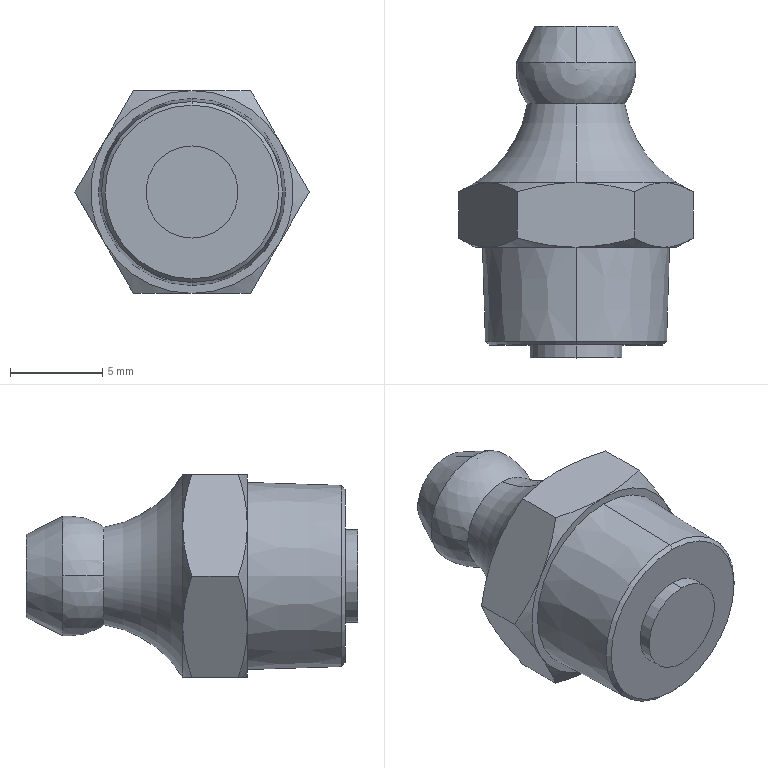Part | SolidWorks | features ICE 9, Revolution 9, Fillet 2 | 2 solids | 43 faces | box 12.702 x 18 x 11 mm | volume 1039 mm3 | cone 20 | plane 11 | cylinder 6 | sphere 4 | torus 2 | commonest cylinder face diameters 1.5 x2 3 x2 5 x2
STEP:
#1=CARTESIAN_POINT('',(0.,13.773,-2.65));
#2=VERTEX_POINT('',#1);
#3=CARTESIAN_POINT('',(-2.65,13.773,0.));
#4=VERTEX_POINT('',#3);
#5=CARTESIAN_POINT('',(0.,13.773,0.));
#6=DIRECTION('',(0.,1.,0.));
#7=DIRECTION('',(0.,0.,1.));
#8=AXIS2_PLACEMENT_3D('',#5,#6,#7);
#9=CIRCLE('',#8,2.65);
#10=EDGE_CURVE('',#2,#4,#9,.T.);
#11=ORIENTED_EDGE('',*,*,#10,.T.);
#12=CARTESIAN_POINT('',(-3.232,16.,0.));
#13=VERTEX_POINT('',#12);
#14=CARTESIAN_POINT('',(0.,15.655,0.));
#15=DIRECTION('',(0.,0.,-1.));
#16=DIRECTION('',(-1.,0.,0.));
#17=AXIS2_PLACEMENT_3D('',#14,#15,#16);
#18=CIRCLE('',#17,3.25);
#19=EDGE_CURVE('',#4,#13,#18,.T.);
#20=ORIENTED_EDGE('',*,*,#19,.T.);
#21=CARTESIAN_POINT('',(0.,16.,-3.232));
#22=VERTEX_POINT('',#21);
#23=CARTESIAN_POINT('',(0.,16.,0.));
#24=DIRECTION('',(0.,1.,0.));
#25=DIRECTION('',(0.,0.,1.));
#26=AXIS2_PLACEMENT_3D('',#23,#24,#25);
#27=CIRCLE('',#26,3.232);
#28=EDGE_CURVE('',#22,#13,#27,.T.);
#29=ORIENTED_EDGE('',*,*,#28,.F.);
#30=CARTESIAN_POINT('',(3.232,16.,0.));
#31=VERTEX_POINT('',#30);
#32=CARTESIAN_POINT('',(0.,16.,0.));
#33=DIRECTION('',(0.,1.,0.));
#34=DIRECTION('',(0.,0.,1.));
#35=AXIS2_PLACEMENT_3D('',#32,#33,#34);
#36=CIRCLE('',#35,3.232);
#37=EDGE_CURVE('',#31,#22,#36,.T.);
#38=ORIENTED_EDGE('',*,*,#37,.F.);
#39=CARTESIAN_POINT('',(2.65,13.773,0.));
#40=VERTEX_POINT('',#39);
#41=CARTESIAN_POINT('',(0.,15.655,0.));
#42=DIRECTION('',(0.,0.,1.));
#43=DIRECTION('',(1.,0.,0.));
#44=AXIS2_PLACEMENT_3D('',#41,#42,#43);
#45=CIRCLE('',#44,3.25);
#46=EDGE_CURVE('',#40,#31,#45,.T.);
#47=ORIENTED_EDGE('',*,*,#46,.F.);
#48=CARTESIAN_POINT('',(0.,13.773,0.));
#49=DIRECTION('',(0.,1.,0.));
#50=DIRECTION('',(0.,0.,1.));
#51=AXIS2_PLACEMENT_3D('',#48,#49,#50);
#52=CIRCLE('',#51,2.65);
#53=EDGE_CURVE('',#40,#2,#52,.T.);
#54=ORIENTED_EDGE('',*,*,#53,.T.);
#55=EDGE_LOOP('',(#11,#20,#29,#38,#47,#54));
#56=FACE_OUTER_BOUND('',#55,.T.);
#57=CARTESIAN_POINT('',(0.,15.655,0.));
#58=DIRECTION('',(0.,0.,-1.));
#59=DIRECTION('',(1.,0.,0.));
#60=AXIS2_PLACEMENT_3D('',#57,#58,#59);
#61=SPHERICAL_SURFACE('',#60,3.25);
#62=ADVANCED_FACE('',(#56),#61,.T.);
#63=CARTESIAN_POINT('',(0.,18.,2.25));
#64=VERTEX_POINT('',#63);
#65=CARTESIAN_POINT('',(0.,18.,-2.25));
#66=VERTEX_POINT('',#65);
#67=CARTESIAN_POINT('',(0.,18.,0.));
#68=DIRECTION('',(0.,1.,0.));
#69=DIRECTION('',(0.,0.,1.));
#70=AXIS2_PLACEMENT_3D('',#67,#68,#69);
#71=CIRCLE('',#70,2.25);
#72=EDGE_CURVE('',#64,#66,#71,.T.);
#73=ORIENTED_EDGE('',*,*,#72,.F.);
#74=CARTESIAN_POINT('',(0.,16.,3.232));
#75=VERTEX_POINT('',#74);
#76=CARTESIAN_POINT('',(0.,18.,2.25));
#77=DIRECTION('',(0.,-0.8977,0.4406));
#78=VECTOR('',#77,1000.);
#79=LINE('',#76,#78);
#80=EDGE_CURVE('',#64,#75,#79,.T.);
#81=ORIENTED_EDGE('',*,*,#80,.T.);
#82=CARTESIAN_POINT('',(0.,16.,0.));
#83=DIRECTION('',(0.,1.,0.));
#84=DIRECTION('',(0.,0.,1.));
#85=AXIS2_PLACEMENT_3D('',#82,#83,#84);
#86=CIRCLE('',#85,3.232);
#87=EDGE_CURVE('',#75,#31,#86,.T.);
#88=ORIENTED_EDGE('',*,*,#87,.T.);
#89=ORIENTED_EDGE('',*,*,#37,.T.);
#90=CARTESIAN_POINT('',(0.,18.,-2.25));
#91=DIRECTION('',(0.,-0.8977,-0.4406));
#92=VECTOR('',#91,1000.);
#93=LINE('',#90,#92);
#94=EDGE_CURVE('',#66,#22,#93,.T.);
#95=ORIENTED_EDGE('',*,*,#94,.F.);
#96=EDGE_LOOP('',(#73,#81,#88,#89,#95));
#97=FACE_OUTER_BOUND('',#96,.T.);
#98=CARTESIAN_POINT('',(0.,18.,0.));
#99=DIRECTION('',(0.,-1.,0.));
#100=DIRECTION('',(0.,0.,-1.));
#101=AXIS2_PLACEMENT_3D('',#98,#99,#100);
#102=CONICAL_SURFACE('',#101,2.25,0.4563);
#103=ADVANCED_FACE('',(#97),#102,.T.);
#104=CARTESIAN_POINT('',(0.,17.689,-0.75));
#105=VERTEX_POINT('',#104);
#106=CARTESIAN_POINT('',(0.,17.689,0.75));
#107=VERTEX_POINT('',#106);
#108=CARTESIAN_POINT('',(0.,17.689,0.));
#109=DIRECTION('',(0.,1.,0.));
#110=DIRECTION('',(0.,0.,1.));
#111=AXIS2_PLACEMENT_3D('',#108,#109,#110);
#112=CIRCLE('',#111,0.75);
#113=EDGE_CURVE('',#105,#107,#112,.T.);
#114=ORIENTED_EDGE('',*,*,#113,.F.);
#115=CARTESIAN_POINT('',(0.,18.,-0.75));
#116=VERTEX_POINT('',#115);
#117=CARTESIAN_POINT('',(0.,18.,-0.75));
#118=DIRECTION('',(0.,1.,0.));
#119=VECTOR('',#118,1000.);
#120=LINE('',#117,#119);
#121=EDGE_CURVE('',#105,#116,#120,.T.);
#122=ORIENTED_EDGE('',*,*,#121,.T.);
#123=CARTESIAN_POINT('',(0.,18.,0.75));
#124=VERTEX_POINT('',#123);
#125=CARTESIAN_POINT('',(0.,18.,0.));
#126=DIRECTION('',(0.,1.,0.));
#127=DIRECTION('',(0.,0.,1.));
#128=AXIS2_PLACEMENT_3D('',#125,#126,#127);
#129=CIRCLE('',#128,0.75);
#130=EDGE_CURVE('',#116,#124,#129,.T.);
#131=ORIENTED_EDGE('',*,*,#130,.T.);
#132=CARTESIAN_POINT('',(0.,18.,0.75));
#133=DIRECTION('',(0.,1.,0.));
#134=VECTOR('',#133,1000.);
#135=LINE('',#132,#134);
#136=EDGE_CURVE('',#107,#124,#135,.T.);
#137=ORIENTED_EDGE('',*,*,#136,.F.);
#138=EDGE_LOOP('',(#114,#122,#131,#137));
#139=FACE_OUTER_BOUND('',#138,.T.);
#140=CARTESIAN_POINT('',(0.,18.,0.));
#141=DIRECTION('',(0.,1.,0.));
#142=DIRECTION('',(0.,0.,1.));
#143=AXIS2_PLACEMENT_3D('',#140,#141,#142);
#144=CYLINDRICAL_SURFACE('',#143,0.75);
#145=ADVANCED_FACE('',(#139),#144,.F.);
#146=ORIENTED_EDGE('',*,*,#113,.T.);
#147=CARTESIAN_POINT('',(0.,16.939,1.5));
#148=VERTEX_POINT('',#147);
#149=CARTESIAN_POINT('',(0.,16.939,1.5));
#150=DIRECTION('',(0.,-0.7071,0.7071));
#151=VECTOR('',#150,1000.);
#152=LINE('',#149,#151);
#153=EDGE_CURVE('',#107,#148,#152,.T.);
#154=ORIENTED_EDGE('',*,*,#153,.T.);
#155=CARTESIAN_POINT('',(0.,16.939,-1.5));
#156=VERTEX_POINT('',#155);
#157=CARTESIAN_POINT('',(0.,16.939,0.));
#158=DIRECTION('',(0.,1.,0.));
#159=DIRECTION('',(0.,0.,1.));
#160=AXIS2_PLACEMENT_3D('',#157,#158,#159);
#161=CIRCLE('',#160,1.5);
#162=EDGE_CURVE('',#156,#148,#161,.T.);
#163=ORIENTED_EDGE('',*,*,#162,.F.);
#164=CARTESIAN_POINT('',(0.,16.939,-1.5));
#165=DIRECTION('',(0.,-0.7071,-0.7071));
#166=VECTOR('',#165,1000.);
#167=LINE('',#164,#166);
#168=EDGE_CURVE('',#105,#156,#167,.T.);
#169=ORIENTED_EDGE('',*,*,#168,.F.);
#170=EDGE_LOOP('',(#146,#154,#163,#169));
#171=FACE_OUTER_BOUND('',#170,.T.);
#172=CARTESIAN_POINT('',(0.,16.939,0.));
#173=DIRECTION('',(0.,-1.,0.));
#174=DIRECTION('',(0.,0.,-1.));
#175=AXIS2_PLACEMENT_3D('',#172,#173,#174);
#176=CONICAL_SURFACE('',#175,1.5,0.7854);
#177=ADVANCED_FACE('',(#171),#176,.F.);
#178=CARTESIAN_POINT('',(0.,9.5,-1.5));
#179=VERTEX_POINT('',#178);
#180=CARTESIAN_POINT('',(0.,9.5,1.5));
#181=VERTEX_POINT('',#180);
#182=CARTESIAN_POINT('',(0.,9.5,0.));
#183=DIRECTION('',(0.,1.,0.));
#184=DIRECTION('',(0.,0.,1.));
#185=AXIS2_PLACEMENT_3D('',#182,#183,#184);
#186=CIRCLE('',#185,1.5);
#187=EDGE_CURVE('',#179,#181,#186,.T.);
#188=ORIENTED_EDGE('',*,*,#187,.F.);
#189=CARTESIAN_POINT('',(0.,18.,-1.5));
#190=DIRECTION('',(0.,1.,0.));
#191=VECTOR('',#190,1000.);
#192=LINE('',#189,#191);
#193=EDGE_CURVE('',#179,#156,#192,.T.);
#194=ORIENTED_EDGE('',*,*,#193,.T.);
#195=ORIENTED_EDGE('',*,*,#162,.T.);
#196=CARTESIAN_POINT('',(0.,18.,1.5));
#197=DIRECTION('',(0.,1.,0.));
#198=VECTOR('',#197,1000.);
#199=LINE('',#196,#198);
#200=EDGE_CURVE('',#181,#148,#199,.T.);
#201=ORIENTED_EDGE('',*,*,#200,.F.);
#202=EDGE_LOOP('',(#188,#194,#195,#201));
#203=FACE_OUTER_BOUND('',#202,.T.);
#204=CARTESIAN_POINT('',(0.,18.,0.));
#205=DIRECTION('',(0.,1.,0.));
#206=DIRECTION('',(0.,0.,1.));
#207=AXIS2_PLACEMENT_3D('',#204,#205,#206);
#208=CYLINDRICAL_SURFACE('',#207,1.5);
#209=ADVANCED_FACE('',(#203),#208,.F.);
#210=ORIENTED_EDGE('',*,*,#10,.F.);
#211=CARTESIAN_POINT('',(0.,9.5,-5.5));
#212=VERTEX_POINT('',#211);
#213=CARTESIAN_POINT('',(0.,14.7,-8.668));
#214=DIRECTION('',(1.,0.,0.));
#215=DIRECTION('',(0.,0.,-1.));
#216=AXIS2_PLACEMENT_3D('',#213,#214,#215);
#217=CIRCLE('',#216,6.089);
#218=EDGE_CURVE('',#2,#212,#217,.T.);
#219=ORIENTED_EDGE('',*,*,#218,.T.);
#220=CARTESIAN_POINT('',(-4.763,9.5,-2.75));
#221=VERTEX_POINT('',#220);
#222=CARTESIAN_POINT('',(0.,9.5,0.));
#223=DIRECTION('',(0.,-1.,0.));
#224=DIRECTION('',(0.,0.,-1.));
#225=AXIS2_PLACEMENT_3D('',#222,#223,#224);
#226=CIRCLE('',#225,5.5);
#227=EDGE_CURVE('',#221,#212,#226,.T.);
#228=ORIENTED_EDGE('',*,*,#227,.F.);
#229=CARTESIAN_POINT('',(-4.763,9.5,2.75));
#230=VERTEX_POINT('',#229);
#231=CARTESIAN_POINT('',(0.,9.5,0.));
#232=DIRECTION('',(0.,-1.,0.));
#233=DIRECTION('',(0.,0.,-1.));
#234=AXIS2_PLACEMENT_3D('',#231,#232,#233);
#235=CIRCLE('',#234,5.5);
#236=EDGE_CURVE('',#230,#221,#235,.T.);
#237=ORIENTED_EDGE('',*,*,#236,.F.);
#238=CARTESIAN_POINT('',(0.,9.5,5.5));
#239=VERTEX_POINT('',#238);
#240=CARTESIAN_POINT('',(0.,9.5,0.));
#241=DIRECTION('',(0.,-1.,0.));
#242=DIRECTION('',(0.,0.,-1.));
#243=AXIS2_PLACEMENT_3D('',#240,#241,#242);
#244=CIRCLE('',#243,5.5);
#245=EDGE_CURVE('',#239,#230,#244,.T.);
#246=ORIENTED_EDGE('',*,*,#245,.F.);
#247=CARTESIAN_POINT('',(0.,13.773,2.65));
#248=VERTEX_POINT('',#247);
#249=CARTESIAN_POINT('',(0.,14.7,8.668));
#250=DIRECTION('',(-1.,0.,0.));
#251=DIRECTION('',(0.,0.,1.));
#252=AXIS2_PLACEMENT_3D('',#249,#250,#251);
#253=CIRCLE('',#252,6.089);
#254=EDGE_CURVE('',#248,#239,#253,.T.);
#255=ORIENTED_EDGE('',*,*,#254,.F.);
#256=CARTESIAN_POINT('',(0.,13.773,0.));
#257=DIRECTION('',(0.,1.,0.));
#258=DIRECTION('',(0.,0.,1.));
#259=AXIS2_PLACEMENT_3D('',#256,#257,#258);
#260=CIRCLE('',#259,2.65);
#261=EDGE_CURVE('',#4,#248,#260,.T.);
#262=ORIENTED_EDGE('',*,*,#261,.F.);
#263=EDGE_LOOP('',(#210,#219,#228,#237,#246,#255,#262));
#264=FACE_OUTER_BOUND('',#263,.T.);
#265=CARTESIAN_POINT('',(0.,14.7,0.));
#266=DIRECTION('',(0.,1.,0.));
#267=DIRECTION('',(0.,0.,1.));
#268=AXIS2_PLACEMENT_3D('',#265,#266,#267);
#269=TOROIDAL_SURFACE('',#268,8.668,6.089);
#270=ADVANCED_FACE('',(#264),#269,.F.);
#271=CARTESIAN_POINT('',(0.,0.9,-4.913));
#272=VERTEX_POINT('',#271);
#273=CARTESIAN_POINT('',(0.,0.9,4.913));
#274=VERTEX_POINT('',#273);
#275=CARTESIAN_POINT('',(0.,0.9,0.));
#276=DIRECTION('',(0.,-1.,0.));
#277=DIRECTION('',(0.,0.,-1.));
#278=AXIS2_PLACEMENT_3D('',#275,#276,#277);
#279=CIRCLE('',#278,4.913);
#280=EDGE_CURVE('',#272,#274,#279,.T.);
#281=ORIENTED_EDGE('',*,*,#280,.F.);
#282=CARTESIAN_POINT('',(0.,6.,-5.072));
#283=VERTEX_POINT('',#282);
#284=CARTESIAN_POINT('',(0.,6.,-5.072));
#285=DIRECTION('',(0.,0.9995,-0.03123));
#286=VECTOR('',#285,1000.);
#287=LINE('',#284,#286);
#288=EDGE_CURVE('',#272,#283,#287,.T.);
#289=ORIENTED_EDGE('',*,*,#288,.T.);
#290=CARTESIAN_POINT('',(0.,6.,5.072));
#291=VERTEX_POINT('',#290);
#292=CARTESIAN_POINT('',(0.,6.,0.));
#293=DIRECTION('',(0.,-1.,0.));
#294=DIRECTION('',(0.,0.,-1.));
#295=AXIS2_PLACEMENT_3D('',#292,#293,#294);
#296=CIRCLE('',#295,5.072);
#297=EDGE_CURVE('',#283,#291,#296,.T.);
#298=ORIENTED_EDGE('',*,*,#297,.T.);
#299=CARTESIAN_POINT('',(0.,6.,5.072));
#300=DIRECTION('',(0.,0.9995,0.03123));
#301=VECTOR('',#300,1000.);
#302=LINE('',#299,#301);
#303=EDGE_CURVE('',#274,#291,#302,.T.);
#304=ORIENTED_EDGE('',*,*,#303,.F.);
#305=EDGE_LOOP('',(#281,#289,#298,#304));
#306=FACE_OUTER_BOUND('',#305,.T.);
#307=CARTESIAN_POINT('',(0.,6.,0.));
#308=DIRECTION('',(0.,1.,0.));
#309=DIRECTION('',(0.,0.,1.));
#310=AXIS2_PLACEMENT_3D('',#307,#308,#309);
#311=CONICAL_SURFACE('',#310,5.072,0.03124);
#312=ADVANCED_FACE('',(#306),#311,.T.);
#313=CARTESIAN_POINT('',(0.,0.7,-4.712));
#314=VERTEX_POINT('',#313);
#315=CARTESIAN_POINT('',(0.,0.7,4.712));
#316=VERTEX_POINT('',#315);
#317=CARTESIAN_POINT('',(0.,0.7,0.));
#318=DIRECTION('',(0.,-1.,0.));
#319=DIRECTION('',(0.,0.,-1.));
#320=AXIS2_PLACEMENT_3D('',#317,#318,#319);
#321=CIRCLE('',#320,4.712);
#322=EDGE_CURVE('',#314,#316,#321,.T.);
#323=ORIENTED_EDGE('',*,*,#322,.F.);
#324=CARTESIAN_POINT('',(0.,0.9,-4.913));
#325=DIRECTION('',(0.,0.7071,-0.7071));
#326=VECTOR('',#325,1000.);
#327=LINE('',#324,#326);
#328=EDGE_CURVE('',#314,#272,#327,.T.);
#329=ORIENTED_EDGE('',*,*,#328,.T.);
#330=ORIENTED_EDGE('',*,*,#280,.T.);
#331=CARTESIAN_POINT('',(0.,0.9,4.913));
#332=DIRECTION('',(0.,0.7071,0.7071));
#333=VECTOR('',#332,1000.);
#334=LINE('',#331,#333);
#335=EDGE_CURVE('',#316,#274,#334,.T.);
#336=ORIENTED_EDGE('',*,*,#335,.F.);
#337=EDGE_LOOP('',(#323,#329,#330,#336));
#338=FACE_OUTER_BOUND('',#337,.T.);
#339=CARTESIAN_POINT('',(0.,0.9,0.));
#340=DIRECTION('',(0.,1.,0.));
#341=DIRECTION('',(0.,0.,1.));
#342=AXIS2_PLACEMENT_3D('',#339,#340,#341);
#343=CONICAL_SURFACE('',#342,4.913,0.7854);
#344=ADVANCED_FACE('',(#338),#343,.T.);
#345=CARTESIAN_POINT('',(0.,0.7,-2.5));
#346=VERTEX_POINT('',#345);
#347=CARTESIAN_POINT('',(0.,0.7,2.5));
#348=VERTEX_POINT('',#347);
#349=CARTESIAN_POINT('',(0.,0.7,0.));
#350=DIRECTION('',(0.,-1.,0.));
#351=DIRECTION('',(0.,0.,-1.));
#352=AXIS2_PLACEMENT_3D('',#349,#350,#351);
#353=CIRCLE('',#352,2.5);
#354=EDGE_CURVE('',#346,#348,#353,.T.);
#355=ORIENTED_EDGE('',*,*,#354,.T.);
#356=CARTESIAN_POINT('',(0.,0.,2.5));
#357=VERTEX_POINT('',#356);
#358=CARTESIAN_POINT('',(0.,0.,2.5));
#359=DIRECTION('',(0.,-1.,0.));
#360=VECTOR('',#359,1000.);
#361=LINE('',#358,#360);
#362=EDGE_CURVE('',#348,#357,#361,.T.);
#363=ORIENTED_EDGE('',*,*,#362,.T.);
#364=CARTESIAN_POINT('',(0.,0.,-2.5));
#365=VERTEX_POINT('',#364);
#366=CARTESIAN_POINT('',(0.,0.,0.));
#367=DIRECTION('',(0.,-1.,0.));
#368=DIRECTION('',(0.,0.,-1.));
#369=AXIS2_PLACEMENT_3D('',#366,#367,#368);
#370=CIRCLE('',#369,2.5);
#371=EDGE_CURVE('',#365,#357,#370,.T.);
#372=ORIENTED_EDGE('',*,*,#371,.F.);
#373=CARTESIAN_POINT('',(0.,0.,-2.5));
#374=DIRECTION('',(0.,-1.,0.));
#375=VECTOR('',#374,1000.);
#376=LINE('',#373,#375);
#377=EDGE_CURVE('',#346,#365,#376,.T.);
#378=ORIENTED_EDGE('',*,*,#377,.F.);
#379=EDGE_LOOP('',(#355,#363,#372,#378));
#380=FACE_OUTER_BOUND('',#379,.T.);
#381=CARTESIAN_POINT('',(0.,0.,0.));
#382=DIRECTION('',(0.,-1.,0.));
#383=DIRECTION('',(0.,0.,-1.));
#384=AXIS2_PLACEMENT_3D('',#381,#382,#383);
#385=CYLINDRICAL_SURFACE('',#384,2.5);
#386=ADVANCED_FACE('',(#380),#385,.T.);
#387=ORIENTED_EDGE('',*,*,#371,.T.);
#388=CARTESIAN_POINT('',(0.,0.,0.));
#389=DIRECTION('',(0.,-1.,0.));
#390=DIRECTION('',(0.,0.,-1.));
#391=AXIS2_PLACEMENT_3D('',#388,#389,#390);
#392=CIRCLE('',#391,2.5);
#393=EDGE_CURVE('',#357,#365,#392,.T.);
#394=ORIENTED_EDGE('',*,*,#393,.T.);
#395=EDGE_LOOP('',(#387,#394));
#396=FACE_OUTER_BOUND('',#395,.T.);
#397=CARTESIAN_POINT('',(0.,0.,0.));
#398=DIRECTION('',(0.,1.,0.));
#399=DIRECTION('',(0.,0.,1.));
#400=AXIS2_PLACEMENT_3D('',#397,#398,#399);
#401=PLANE('',#400);
#402=ADVANCED_FACE('',(#396),#401,.F.);
#403=ORIENTED_EDGE('',*,*,#362,.F.);
#404=CARTESIAN_POINT('',(0.,0.7,0.));
#405=DIRECTION('',(0.,-1.,0.));
#406=DIRECTION('',(0.,0.,-1.));
#407=AXIS2_PLACEMENT_3D('',#404,#405,#406);
#408=CIRCLE('',#407,2.5);
#409=EDGE_CURVE('',#348,#346,#408,.T.);
#410=ORIENTED_EDGE('',*,*,#409,.T.);
#411=ORIENTED_EDGE('',*,*,#377,.T.);
#412=ORIENTED_EDGE('',*,*,#393,.F.);
#413=EDGE_LOOP('',(#403,#410,#411,#412));
#414=FACE_OUTER_BOUND('',#413,.T.);
#415=CARTESIAN_POINT('',(0.,0.,0.));
#416=DIRECTION('',(0.,-1.,0.));
#417=DIRECTION('',(0.,0.,-1.));
#418=AXIS2_PLACEMENT_3D('',#415,#416,#417);
#419=CYLINDRICAL_SURFACE('',#418,2.5);
#420=ADVANCED_FACE('',(#414),#419,.T.);
#421=ORIENTED_EDGE('',*,*,#354,.F.);
#422=ORIENTED_EDGE('',*,*,#409,.F.);
#423=EDGE_LOOP('',(#421,#422));
#424=FACE_BOUND('',#423,.T.);
#425=CARTESIAN_POINT('',(0.,0.7,0.));
#426=DIRECTION('',(0.,-1.,0.));
#427=DIRECTION('',(0.,0.,-1.));
#428=AXIS2_PLACEMENT_3D('',#425,#426,#427);
#429=CIRCLE('',#428,4.712);
#430=EDGE_CURVE('',#316,#314,#429,.T.);
#431=ORIENTED_EDGE('',*,*,#430,.T.);
#432=ORIENTED_EDGE('',*,*,#322,.T.);
#433=EDGE_LOOP('',(#431,#432));
#434=FACE_OUTER_BOUND('',#433,.T.);
#435=CARTESIAN_POINT('',(2.5,0.7,0.));
#436=DIRECTION('',(0.,1.,0.));
#437=DIRECTION('',(0.,0.,1.));
#438=AXIS2_PLACEMENT_3D('',#435,#436,#437);
#439=PLANE('',#438);
#440=ADVANCED_FACE('',(#424,#434),#439,.F.);
#441=ORIENTED_EDGE('',*,*,#328,.F.);
#442=ORIENTED_EDGE('',*,*,#430,.F.);
#443=ORIENTED_EDGE('',*,*,#335,.T.);
#444=CARTESIAN_POINT('',(0.,0.9,0.));
#445=DIRECTION('',(0.,-1.,0.));
#446=DIRECTION('',(0.,0.,-1.));
#447=AXIS2_PLACEMENT_3D('',#444,#445,#446);
#448=CIRCLE('',#447,4.913);
#449=EDGE_CURVE('',#274,#272,#448,.T.);
#450=ORIENTED_EDGE('',*,*,#449,.T.);
#451=EDGE_LOOP('',(#441,#442,#443,#450));
#452=FACE_OUTER_BOUND('',#451,.T.);
#453=CARTESIAN_POINT('',(0.,0.9,0.));
#454=DIRECTION('',(0.,1.,0.));
#455=DIRECTION('',(0.,0.,1.));
#456=AXIS2_PLACEMENT_3D('',#453,#454,#455);
#457=CONICAL_SURFACE('',#456,4.913,0.7854);
#458=ADVANCED_FACE('',(#452),#457,.T.);
#459=ORIENTED_EDGE('',*,*,#288,.F.);
#460=ORIENTED_EDGE('',*,*,#449,.F.);
#461=ORIENTED_EDGE('',*,*,#303,.T.);
#462=CARTESIAN_POINT('',(0.,6.,0.));
#463=DIRECTION('',(0.,-1.,0.));
#464=DIRECTION('',(0.,0.,-1.));
#465=AXIS2_PLACEMENT_3D('',#462,#463,#464);
#466=CIRCLE('',#465,5.072);
#467=EDGE_CURVE('',#291,#283,#466,.T.);
#468=ORIENTED_EDGE('',*,*,#467,.T.);
#469=EDGE_LOOP('',(#459,#460,#461,#468));
#470=FACE_OUTER_BOUND('',#469,.T.);
#471=CARTESIAN_POINT('',(0.,6.,0.));
#472=DIRECTION('',(0.,1.,0.));
#473=DIRECTION('',(0.,0.,1.));
#474=AXIS2_PLACEMENT_3D('',#471,#472,#473);
#475=CONICAL_SURFACE('',#474,5.072,0.03124);
#476=ADVANCED_FACE('',(#470),#475,.T.);
#477=ORIENTED_EDGE('',*,*,#467,.F.);
#478=ORIENTED_EDGE('',*,*,#297,.F.);
#479=EDGE_LOOP('',(#477,#478));
#480=FACE_BOUND('',#479,.T.);
#481=CARTESIAN_POINT('',(0.,6.,5.5));
#482=VERTEX_POINT('',#481);
#483=CARTESIAN_POINT('',(4.763,6.,2.75));
#484=VERTEX_POINT('',#483);
#485=CARTESIAN_POINT('',(0.,6.,0.));
#486=DIRECTION('',(0.,1.,0.));
#487=DIRECTION('',(0.,0.,1.));
#488=AXIS2_PLACEMENT_3D('',#485,#486,#487);
#489=CIRCLE('',#488,5.5);
#490=EDGE_CURVE('',#482,#484,#489,.T.);
#491=ORIENTED_EDGE('',*,*,#490,.F.);
#492=CARTESIAN_POINT('',(-4.763,6.,2.75));
#493=VERTEX_POINT('',#492);
#494=CARTESIAN_POINT('',(0.,6.,0.));
#495=DIRECTION('',(0.,-1.,0.));
#496=DIRECTION('',(0.,0.,1.));
#497=AXIS2_PLACEMENT_3D('',#494,#495,#496);
#498=CIRCLE('',#497,5.5);
#499=EDGE_CURVE('',#482,#493,#498,.T.);
#500=ORIENTED_EDGE('',*,*,#499,.T.);
#501=CARTESIAN_POINT('',(-4.763,6.,-2.75));
#502=VERTEX_POINT('',#501);
#503=CARTESIAN_POINT('',(0.,6.,0.));
#504=DIRECTION('',(0.,-1.,0.));
#505=DIRECTION('',(0.,0.,1.));
#506=AXIS2_PLACEMENT_3D('',#503,#504,#505);
#507=CIRCLE('',#506,5.5);
#508=EDGE_CURVE('',#493,#502,#507,.T.);
#509=ORIENTED_EDGE('',*,*,#508,.T.);
#510=CARTESIAN_POINT('',(0.,6.,-5.5));
#511=VERTEX_POINT('',#510);
#512=CARTESIAN_POINT('',(0.,6.,0.));
#513=DIRECTION('',(0.,-1.,0.));
#514=DIRECTION('',(0.,0.,1.));
#515=AXIS2_PLACEMENT_3D('',#512,#513,#514);
#516=CIRCLE('',#515,5.5);
#517=EDGE_CURVE('',#502,#511,#516,.T.);
#518=ORIENTED_EDGE('',*,*,#517,.T.);
#519=CARTESIAN_POINT('',(4.763,6.,-2.75));
#520=VERTEX_POINT('',#519);
#521=CARTESIAN_POINT('',(0.,6.,0.));
#522=DIRECTION('',(0.,-1.,0.));
#523=DIRECTION('',(0.,0.,1.));
#524=AXIS2_PLACEMENT_3D('',#521,#522,#523);
#525=CIRCLE('',#524,5.5);
#526=EDGE_CURVE('',#511,#520,#525,.T.);
#527=ORIENTED_EDGE('',*,*,#526,.T.);
#528=CARTESIAN_POINT('',(0.,6.,0.));
#529=DIRECTION('',(0.,-1.,0.));
#530=DIRECTION('',(0.,0.,1.));
#531=AXIS2_PLACEMENT_3D('',#528,#529,#530);
#532=CIRCLE('',#531,5.5);
#533=EDGE_CURVE('',#520,#484,#532,.T.);
#534=ORIENTED_EDGE('',*,*,#533,.T.);
#535=EDGE_LOOP('',(#491,#500,#509,#518,#527,#534));
#536=FACE_OUTER_BOUND('',#535,.T.);
#537=CARTESIAN_POINT('',(5.072,6.,0.));
#538=DIRECTION('',(0.,1.,0.));
#539=DIRECTION('',(0.,0.,1.));
#540=AXIS2_PLACEMENT_3D('',#537,#538,#539);
#541=PLANE('',#540);
#542=ADVANCED_FACE('',(#480,#536),#541,.F.);
#543=CARTESIAN_POINT('',(3.175,6.491,5.5));
#544=VERTEX_POINT('',#543);
#545=CARTESIAN_POINT('',(4.763,6.,2.75));
#546=CARTESIAN_POINT('',(4.628,6.,2.983));
#547=CARTESIAN_POINT('',(4.493,6.012,3.218));
#548=CARTESIAN_POINT('',(4.225,6.057,3.682));
#549=CARTESIAN_POINT('',(4.092,6.09,3.912));
#550=CARTESIAN_POINT('',(3.696,6.218,4.599));
#551=CARTESIAN_POINT('',(3.435,6.342,5.051));
#552=CARTESIAN_POINT('',(3.175,6.491,5.5));
#553=B_SPLINE_CURVE_WITH_KNOTS('',3,(#545,#546,#547,#548,#549,#550,#551,#552),.UNSPECIFIED.,.F.,.F.,(4,2,2,4),(0.003213,0.004014,0.004814,0.006414),.UNSPECIFIED.);
#554=EDGE_CURVE('',#484,#544,#553,.T.);
#555=ORIENTED_EDGE('',*,*,#554,.T.);
#556=CARTESIAN_POINT('',(3.175,6.491,5.5));
#557=CARTESIAN_POINT('',(2.662,6.343,5.5));
#558=CARTESIAN_POINT('',(2.142,6.22,5.5));
#559=CARTESIAN_POINT('',(1.082,6.048,5.5));
#560=CARTESIAN_POINT('',(0.5376,6.,5.5));
#561=CARTESIAN_POINT('',(0.,6.,5.5));
#562=B_SPLINE_CURVE_WITH_KNOTS('',3,(#556,#557,#558,#559,#560,#561),.UNSPECIFIED.,.F.,.F.,(4,2,4),(0.01649,0.01809,0.0197),.UNSPECIFIED.);
#563=EDGE_CURVE('',#544,#482,#562,.T.);
#564=ORIENTED_EDGE('',*,*,#563,.T.);
#565=ORIENTED_EDGE('',*,*,#490,.T.);
#566=EDGE_LOOP('',(#555,#564,#565));
#567=FACE_OUTER_BOUND('',#566,.T.);
#568=CARTESIAN_POINT('',(0.,6.,0.));
#569=DIRECTION('',(0.,1.,0.));
#570=DIRECTION('',(0.,0.,1.));
#571=AXIS2_PLACEMENT_3D('',#568,#569,#570);
#572=CONICAL_SURFACE('',#571,5.5,1.047);
#573=ADVANCED_FACE('',(#567),#572,.T.);
#574=CARTESIAN_POINT('',(6.351,6.491,0.));
#575=VERTEX_POINT('',#574);
#576=CARTESIAN_POINT('',(4.763,6.,-2.75));
#577=CARTESIAN_POINT('',(4.898,6.,-2.517));
#578=CARTESIAN_POINT('',(5.033,6.012,-2.282));
#579=CARTESIAN_POINT('',(5.301,6.057,-1.818));
#580=CARTESIAN_POINT('',(5.434,6.09,-1.588));
#581=CARTESIAN_POINT('',(5.831,6.218,-0.9012));
#582=CARTESIAN_POINT('',(6.092,6.342,-0.4487));
#583=CARTESIAN_POINT('',(6.351,6.491,0.));
#584=B_SPLINE_CURVE_WITH_KNOTS('',3,(#576,#577,#578,#579,#580,#581,#582,#583),.UNSPECIFIED.,.F.,.F.,(4,2,2,4),(0.003213,0.004014,0.004814,0.006414),.UNSPECIFIED.);
#585=EDGE_CURVE('',#520,#575,#584,.T.);
#586=ORIENTED_EDGE('',*,*,#585,.T.);
#587=CARTESIAN_POINT('',(6.351,6.491,0.));
#588=CARTESIAN_POINT('',(5.831,6.191,0.8997));
#589=CARTESIAN_POINT('',(5.304,6.,1.813));
#590=CARTESIAN_POINT('',(4.763,6.,2.75));
#591=B_SPLINE_CURVE_WITH_KNOTS('',3,(#587,#588,#589,#590),.UNSPECIFIED.,.F.,.F.,(4,4),(0.000000238,0.003213),.UNSPECIFIED.);
#592=EDGE_CURVE('',#575,#484,#591,.T.);
#593=ORIENTED_EDGE('',*,*,#592,.T.);
#594=ORIENTED_EDGE('',*,*,#533,.F.);
#595=EDGE_LOOP('',(#586,#593,#594));
#596=FACE_OUTER_BOUND('',#595,.T.);
#597=CARTESIAN_POINT('',(0.,6.,0.));
#598=DIRECTION('',(0.,1.,0.));
#599=DIRECTION('',(0.,0.,1.));
#600=AXIS2_PLACEMENT_3D('',#597,#598,#599);
#601=CONICAL_SURFACE('',#600,5.5,1.047);
#602=ADVANCED_FACE('',(#596),#601,.T.);
#603=CARTESIAN_POINT('',(3.175,6.491,-5.5));
#604=VERTEX_POINT('',#603);
#605=CARTESIAN_POINT('',(0.,6.,-5.5));
#606=CARTESIAN_POINT('',(0.5376,6.,-5.5));
#607=CARTESIAN_POINT('',(1.082,6.048,-5.5));
#608=CARTESIAN_POINT('',(2.142,6.22,-5.5));
#609=CARTESIAN_POINT('',(2.662,6.343,-5.5));
#610=CARTESIAN_POINT('',(3.175,6.491,-5.5));
#611=B_SPLINE_CURVE_WITH_KNOTS('',3,(#605,#606,#607,#608,#609,#610),.UNSPECIFIED.,.F.,.F.,(4,2,4),(0.009075,0.01068,0.01229),.UNSPECIFIED.);
#612=EDGE_CURVE('',#511,#604,#611,.T.);
#613=ORIENTED_EDGE('',*,*,#612,.T.);
#614=CARTESIAN_POINT('',(3.175,6.491,-5.5));
#615=CARTESIAN_POINT('',(3.695,6.191,-4.6));
#616=CARTESIAN_POINT('',(4.222,6.,-3.687));
#617=CARTESIAN_POINT('',(4.763,6.,-2.75));
#618=B_SPLINE_CURVE_WITH_KNOTS('',3,(#614,#615,#616,#617),.UNSPECIFIED.,.F.,.F.,(4,4),(0.000000238,0.003213),.UNSPECIFIED.);
#619=EDGE_CURVE('',#604,#520,#618,.T.);
#620=ORIENTED_EDGE('',*,*,#619,.T.);
#621=ORIENTED_EDGE('',*,*,#526,.F.);
#622=EDGE_LOOP('',(#613,#620,#621));
#623=FACE_OUTER_BOUND('',#622,.T.);
#624=CARTESIAN_POINT('',(0.,6.,0.));
#625=DIRECTION('',(0.,1.,0.));
#626=DIRECTION('',(0.,0.,1.));
#627=AXIS2_PLACEMENT_3D('',#624,#625,#626);
#628=CONICAL_SURFACE('',#627,5.5,1.047);
#629=ADVANCED_FACE('',(#623),#628,.T.);
#630=CARTESIAN_POINT('',(-3.175,6.491,-5.5));
#631=VERTEX_POINT('',#630);
#632=CARTESIAN_POINT('',(-3.175,6.491,-5.5));
#633=CARTESIAN_POINT('',(-2.658,6.342,-5.5));
#634=CARTESIAN_POINT('',(-2.13,6.217,-5.5));
#635=CARTESIAN_POINT('',(-1.07,6.046,-5.5));
#636=CARTESIAN_POINT('',(-0.5372,6.,-5.5));
#637=CARTESIAN_POINT('',(0.,6.,-5.5));
#638=B_SPLINE_CURVE_WITH_KNOTS('',3,(#632,#633,#634,#635,#636,#637),.UNSPECIFIED.,.F.,.F.,(4,2,4),(0.005861,0.007468,0.009075),.UNSPECIFIED.);
#639=EDGE_CURVE('',#631,#511,#638,.T.);
#640=ORIENTED_EDGE('',*,*,#639,.T.);
#641=ORIENTED_EDGE('',*,*,#517,.F.);
#642=CARTESIAN_POINT('',(-4.763,6.,-2.75));
#643=CARTESIAN_POINT('',(-4.628,6.,-2.983));
#644=CARTESIAN_POINT('',(-4.493,6.012,-3.218));
#645=CARTESIAN_POINT('',(-4.225,6.057,-3.682));
#646=CARTESIAN_POINT('',(-4.092,6.09,-3.912));
#647=CARTESIAN_POINT('',(-3.696,6.218,-4.599));
#648=CARTESIAN_POINT('',(-3.435,6.342,-5.051));
#649=CARTESIAN_POINT('',(-3.175,6.491,-5.5));
#650=B_SPLINE_CURVE_WITH_KNOTS('',3,(#642,#643,#644,#645,#646,#647,#648,#649),.UNSPECIFIED.,.F.,.F.,(4,2,2,4),(0.003213,0.004014,0.004814,0.006414),.UNSPECIFIED.);
#651=EDGE_CURVE('',#502,#631,#650,.T.);
#652=ORIENTED_EDGE('',*,*,#651,.T.);
#653=EDGE_LOOP('',(#640,#641,#652));
#654=FACE_OUTER_BOUND('',#653,.T.);
#655=CARTESIAN_POINT('',(0.,6.,0.));
#656=DIRECTION('',(0.,1.,0.));
#657=DIRECTION('',(0.,0.,1.));
#658=AXIS2_PLACEMENT_3D('',#655,#656,#657);
#659=CONICAL_SURFACE('',#658,5.5,1.047);
#660=ADVANCED_FACE('',(#654),#659,.T.);
#661=CARTESIAN_POINT('',(-6.351,6.491,0.));
#662=VERTEX_POINT('',#661);
#663=CARTESIAN_POINT('',(-4.763,6.,2.75));
#664=CARTESIAN_POINT('',(-4.898,6.,2.517));
#665=CARTESIAN_POINT('',(-5.033,6.012,2.282));
#666=CARTESIAN_POINT('',(-5.301,6.057,1.818));
#667=CARTESIAN_POINT('',(-5.434,6.09,1.588));
#668=CARTESIAN_POINT('',(-5.831,6.218,0.9012));
#669=CARTESIAN_POINT('',(-6.092,6.342,0.4487));
#670=CARTESIAN_POINT('',(-6.351,6.491,0.));
#671=B_SPLINE_CURVE_WITH_KNOTS('',3,(#663,#664,#665,#666,#667,#668,#669,#670),.UNSPECIFIED.,.F.,.F.,(4,2,2,4),(0.003213,0.004014,0.004814,0.006414),.UNSPECIFIED.);
#672=EDGE_CURVE('',#493,#662,#671,.T.);
#673=ORIENTED_EDGE('',*,*,#672,.T.);
#674=CARTESIAN_POINT('',(-6.351,6.491,0.));
#675=CARTESIAN_POINT('',(-5.831,6.191,-0.8997));
#676=CARTESIAN_POINT('',(-5.304,6.,-1.813));
#677=CARTESIAN_POINT('',(-4.763,6.,-2.75));
#678=B_SPLINE_CURVE_WITH_KNOTS('',3,(#674,#675,#676,#677),.UNSPECIFIED.,.F.,.F.,(4,4),(0.000000238,0.003213),.UNSPECIFIED.);
#679=EDGE_CURVE('',#662,#502,#678,.T.);
#680=ORIENTED_EDGE('',*,*,#679,.T.);
#681=ORIENTED_EDGE('',*,*,#508,.F.);
#682=EDGE_LOOP('',(#673,#680,#681));
#683=FACE_OUTER_BOUND('',#682,.T.);
#684=CARTESIAN_POINT('',(0.,6.,0.));
#685=DIRECTION('',(0.,1.,0.));
#686=DIRECTION('',(0.,0.,1.));
#687=AXIS2_PLACEMENT_3D('',#684,#685,#686);
#688=CONICAL_SURFACE('',#687,5.5,1.047);
#689=ADVANCED_FACE('',(#683),#688,.T.);
#690=CARTESIAN_POINT('',(-3.175,6.491,5.5));
#691=VERTEX_POINT('',#690);
#692=CARTESIAN_POINT('',(0.,6.,5.5));
#693=CARTESIAN_POINT('',(-0.5372,6.,5.5));
#694=CARTESIAN_POINT('',(-1.07,6.046,5.5));
#695=CARTESIAN_POINT('',(-2.13,6.217,5.5));
#696=CARTESIAN_POINT('',(-2.658,6.342,5.5));
#697=CARTESIAN_POINT('',(-3.175,6.491,5.5));
#698=B_SPLINE_CURVE_WITH_KNOTS('',3,(#692,#693,#694,#695,#696,#697),.UNSPECIFIED.,.F.,.F.,(4,2,4),(0.0197,0.02131,0.02292),.UNSPECIFIED.);
#699=EDGE_CURVE('',#482,#691,#698,.T.);
#700=ORIENTED_EDGE('',*,*,#699,.T.);
#701=CARTESIAN_POINT('',(-3.175,6.491,5.5));
#702=CARTESIAN_POINT('',(-3.695,6.191,4.6));
#703=CARTESIAN_POINT('',(-4.222,6.,3.687));
#704=CARTESIAN_POINT('',(-4.763,6.,2.75));
#705=B_SPLINE_CURVE_WITH_KNOTS('',3,(#701,#702,#703,#704),.UNSPECIFIED.,.F.,.F.,(4,4),(0.000000238,0.003213),.UNSPECIFIED.);
#706=EDGE_CURVE('',#691,#493,#705,.T.);
#707=ORIENTED_EDGE('',*,*,#706,.T.);
#708=ORIENTED_EDGE('',*,*,#499,.F.);
#709=EDGE_LOOP('',(#700,#707,#708));
#710=FACE_OUTER_BOUND('',#709,.T.);
#711=CARTESIAN_POINT('',(0.,6.,0.));
#712=DIRECTION('',(0.,1.,0.));
#713=DIRECTION('',(0.,0.,1.));
#714=AXIS2_PLACEMENT_3D('',#711,#712,#713);
#715=CONICAL_SURFACE('',#714,5.5,1.047);
#716=ADVANCED_FACE('',(#710),#715,.T.);
#717=CARTESIAN_POINT('',(4.763,9.5,-2.75));
#718=VERTEX_POINT('',#717);
#719=CARTESIAN_POINT('',(0.,9.5,0.));
#720=DIRECTION('',(0.,-1.,0.));
#721=DIRECTION('',(0.,0.,-1.));
#722=AXIS2_PLACEMENT_3D('',#719,#720,#721);
#723=CIRCLE('',#722,5.5);
#724=EDGE_CURVE('',#212,#718,#723,.T.);
#725=ORIENTED_EDGE('',*,*,#724,.T.);
#726=CARTESIAN_POINT('',(3.175,9.009,-5.5));
#727=VERTEX_POINT('',#726);
#728=CARTESIAN_POINT('',(3.175,9.009,-5.5));
#729=CARTESIAN_POINT('',(3.695,9.309,-4.6));
#730=CARTESIAN_POINT('',(4.222,9.5,-3.687));
#731=CARTESIAN_POINT('',(4.763,9.5,-2.75));
#732=B_SPLINE_CURVE_WITH_KNOTS('',3,(#728,#729,#730,#731),.UNSPECIFIED.,.F.,.F.,(4,4),(0.000000238,0.003213),.UNSPECIFIED.);
#733=EDGE_CURVE('',#727,#718,#732,.T.);
#734=ORIENTED_EDGE('',*,*,#733,.F.);
#735=CARTESIAN_POINT('',(0.,9.5,-5.5));
#736=CARTESIAN_POINT('',(0.5376,9.5,-5.5));
#737=CARTESIAN_POINT('',(1.082,9.452,-5.5));
#738=CARTESIAN_POINT('',(2.142,9.28,-5.5));
#739=CARTESIAN_POINT('',(2.662,9.157,-5.5));
#740=CARTESIAN_POINT('',(3.175,9.009,-5.5));
#741=B_SPLINE_CURVE_WITH_KNOTS('',3,(#735,#736,#737,#738,#739,#740),.UNSPECIFIED.,.F.,.F.,(4,2,4),(0.009075,0.01068,0.01229),.UNSPECIFIED.);
#742=EDGE_CURVE('',#212,#727,#741,.T.);
#743=ORIENTED_EDGE('',*,*,#742,.F.);
#744=EDGE_LOOP('',(#725,#734,#743));
#745=FACE_OUTER_BOUND('',#744,.T.);
#746=CARTESIAN_POINT('',(0.,9.5,0.));
#747=DIRECTION('',(0.,-1.,0.));
#748=DIRECTION('',(0.,0.,1.));
#749=AXIS2_PLACEMENT_3D('',#746,#747,#748);
#750=CONICAL_SURFACE('',#749,5.5,1.047);
#751=ADVANCED_FACE('',(#745),#750,.T.);
#752=CARTESIAN_POINT('',(4.763,9.5,2.75));
#753=VERTEX_POINT('',#752);
#754=CARTESIAN_POINT('',(0.,9.5,0.));
#755=DIRECTION('',(0.,-1.,0.));
#756=DIRECTION('',(0.,0.,-1.));
#757=AXIS2_PLACEMENT_3D('',#754,#755,#756);
#758=CIRCLE('',#757,5.5);
#759=EDGE_CURVE('',#718,#753,#758,.T.);
#760=ORIENTED_EDGE('',*,*,#759,.T.);
#761=CARTESIAN_POINT('',(6.351,9.009,0.));
#762=VERTEX_POINT('',#761);
#763=CARTESIAN_POINT('',(6.351,9.009,0.));
#764=CARTESIAN_POINT('',(5.831,9.309,0.8997));
#765=CARTESIAN_POINT('',(5.304,9.5,1.813));
#766=CARTESIAN_POINT('',(4.763,9.5,2.75));
#767=B_SPLINE_CURVE_WITH_KNOTS('',3,(#763,#764,#765,#766),.UNSPECIFIED.,.F.,.F.,(4,4),(0.000000238,0.003213),.UNSPECIFIED.);
#768=EDGE_CURVE('',#762,#753,#767,.T.);
#769=ORIENTED_EDGE('',*,*,#768,.F.);
#770=CARTESIAN_POINT('',(4.763,9.5,-2.75));
#771=CARTESIAN_POINT('',(4.898,9.5,-2.517));
#772=CARTESIAN_POINT('',(5.033,9.488,-2.282));
#773=CARTESIAN_POINT('',(5.301,9.443,-1.818));
#774=CARTESIAN_POINT('',(5.434,9.41,-1.588));
#775=CARTESIAN_POINT('',(5.831,9.282,-0.9012));
#776=CARTESIAN_POINT('',(6.092,9.158,-0.4487));
#777=CARTESIAN_POINT('',(6.351,9.009,0.));
#778=B_SPLINE_CURVE_WITH_KNOTS('',3,(#770,#771,#772,#773,#774,#775,#776,#777),.UNSPECIFIED.,.F.,.F.,(4,2,2,4),(0.003213,0.004014,0.004814,0.006414),.UNSPECIFIED.);
#779=EDGE_CURVE('',#718,#762,#778,.T.);
#780=ORIENTED_EDGE('',*,*,#779,.F.);
#781=EDGE_LOOP('',(#760,#769,#780));
#782=FACE_OUTER_BOUND('',#781,.T.);
#783=CARTESIAN_POINT('',(0.,9.5,0.));
#784=DIRECTION('',(0.,-1.,0.));
#785=DIRECTION('',(0.,0.,1.));
#786=AXIS2_PLACEMENT_3D('',#783,#784,#785);
#787=CONICAL_SURFACE('',#786,5.5,1.047);
#788=ADVANCED_FACE('',(#782),#787,.T.);
#789=CARTESIAN_POINT('',(0.,9.5,0.));
#790=DIRECTION('',(0.,1.,0.));
#791=DIRECTION('',(0.,0.,1.));
#792=AXIS2_PLACEMENT_3D('',#789,#790,#791);
#793=CIRCLE('',#792,5.5);
#794=EDGE_CURVE('',#239,#753,#793,.T.);
#795=ORIENTED_EDGE('',*,*,#794,.F.);
#796=CARTESIAN_POINT('',(3.175,9.009,5.5));
#797=VERTEX_POINT('',#796);
#798=CARTESIAN_POINT('',(3.175,9.009,5.5));
#799=CARTESIAN_POINT('',(2.662,9.157,5.5));
#800=CARTESIAN_POINT('',(2.142,9.28,5.5));
#801=CARTESIAN_POINT('',(1.082,9.452,5.5));
#802=CARTESIAN_POINT('',(0.5376,9.5,5.5));
#803=CARTESIAN_POINT('',(0.,9.5,5.5));
#804=B_SPLINE_CURVE_WITH_KNOTS('',3,(#798,#799,#800,#801,#802,#803),.UNSPECIFIED.,.F.,.F.,(4,2,4),(0.01649,0.01809,0.0197),.UNSPECIFIED.);
#805=EDGE_CURVE('',#797,#239,#804,.T.);
#806=ORIENTED_EDGE('',*,*,#805,.F.);
#807=CARTESIAN_POINT('',(4.763,9.5,2.75));
#808=CARTESIAN_POINT('',(4.628,9.5,2.983));
#809=CARTESIAN_POINT('',(4.493,9.488,3.218));
#810=CARTESIAN_POINT('',(4.225,9.443,3.682));
#811=CARTESIAN_POINT('',(4.092,9.41,3.912));
#812=CARTESIAN_POINT('',(3.696,9.282,4.599));
#813=CARTESIAN_POINT('',(3.435,9.158,5.051));
#814=CARTESIAN_POINT('',(3.175,9.009,5.5));
#815=B_SPLINE_CURVE_WITH_KNOTS('',3,(#807,#808,#809,#810,#811,#812,#813,#814),.UNSPECIFIED.,.F.,.F.,(4,2,2,4),(0.003213,0.004014,0.004814,0.006414),.UNSPECIFIED.);
#816=EDGE_CURVE('',#753,#797,#815,.T.);
#817=ORIENTED_EDGE('',*,*,#816,.F.);
#818=EDGE_LOOP('',(#795,#806,#817));
#819=FACE_OUTER_BOUND('',#818,.T.);
#820=CARTESIAN_POINT('',(0.,9.5,0.));
#821=DIRECTION('',(0.,-1.,0.));
#822=DIRECTION('',(0.,0.,1.));
#823=AXIS2_PLACEMENT_3D('',#820,#821,#822);
#824=CONICAL_SURFACE('',#823,5.5,1.047);
#825=ADVANCED_FACE('',(#819),#824,.T.);
#826=ORIENTED_EDGE('',*,*,#245,.T.);
#827=CARTESIAN_POINT('',(-3.175,9.009,5.5));
#828=VERTEX_POINT('',#827);
#829=CARTESIAN_POINT('',(-3.175,9.009,5.5));
#830=CARTESIAN_POINT('',(-3.695,9.309,4.6));
#831=CARTESIAN_POINT('',(-4.222,9.5,3.687));
#832=CARTESIAN_POINT('',(-4.763,9.5,2.75));
#833=B_SPLINE_CURVE_WITH_KNOTS('',3,(#829,#830,#831,#832),.UNSPECIFIED.,.F.,.F.,(4,4),(0.000000238,0.003213),.UNSPECIFIED.);
#834=EDGE_CURVE('',#828,#230,#833,.T.);
#835=ORIENTED_EDGE('',*,*,#834,.F.);
#836=CARTESIAN_POINT('',(0.,9.5,5.5));
#837=CARTESIAN_POINT('',(-0.5372,9.5,5.5));
#838=CARTESIAN_POINT('',(-1.07,9.454,5.5));
#839=CARTESIAN_POINT('',(-2.13,9.283,5.5));
#840=CARTESIAN_POINT('',(-2.658,9.158,5.5));
#841=CARTESIAN_POINT('',(-3.175,9.009,5.5));
#842=B_SPLINE_CURVE_WITH_KNOTS('',3,(#836,#837,#838,#839,#840,#841),.UNSPECIFIED.,.F.,.F.,(4,2,4),(0.0197,0.02131,0.02292),.UNSPECIFIED.);
#843=EDGE_CURVE('',#239,#828,#842,.T.);
#844=ORIENTED_EDGE('',*,*,#843,.F.);
#845=EDGE_LOOP('',(#826,#835,#844));
#846=FACE_OUTER_BOUND('',#845,.T.);
#847=CARTESIAN_POINT('',(0.,9.5,0.));
#848=DIRECTION('',(0.,-1.,0.));
#849=DIRECTION('',(0.,0.,1.));
#850=AXIS2_PLACEMENT_3D('',#847,#848,#849);
#851=CONICAL_SURFACE('',#850,5.5,1.047);
#852=ADVANCED_FACE('',(#846),#851,.T.);
#853=CARTESIAN_POINT('',(-3.175,9.009,-5.5));
#854=VERTEX_POINT('',#853);
#855=CARTESIAN_POINT('',(-4.763,9.5,-2.75));
#856=CARTESIAN_POINT('',(-4.628,9.5,-2.983));
#857=CARTESIAN_POINT('',(-4.493,9.488,-3.218));
#858=CARTESIAN_POINT('',(-4.225,9.443,-3.682));
#859=CARTESIAN_POINT('',(-4.092,9.41,-3.912));
#860=CARTESIAN_POINT('',(-3.696,9.282,-4.599));
#861=CARTESIAN_POINT('',(-3.435,9.158,-5.051));
#862=CARTESIAN_POINT('',(-3.175,9.009,-5.5));
#863=B_SPLINE_CURVE_WITH_KNOTS('',3,(#855,#856,#857,#858,#859,#860,#861,#862),.UNSPECIFIED.,.F.,.F.,(4,2,2,4),(0.003213,0.004014,0.004814,0.006414),.UNSPECIFIED.);
#864=EDGE_CURVE('',#221,#854,#863,.T.);
#865=ORIENTED_EDGE('',*,*,#864,.F.);
#866=ORIENTED_EDGE('',*,*,#227,.T.);
#867=CARTESIAN_POINT('',(-3.175,9.009,-5.5));
#868=CARTESIAN_POINT('',(-2.658,9.158,-5.5));
#869=CARTESIAN_POINT('',(-2.13,9.283,-5.5));
#870=CARTESIAN_POINT('',(-1.07,9.454,-5.5));
#871=CARTESIAN_POINT('',(-0.5372,9.5,-5.5));
#872=CARTESIAN_POINT('',(0.,9.5,-5.5));
#873=B_SPLINE_CURVE_WITH_KNOTS('',3,(#867,#868,#869,#870,#871,#872),.UNSPECIFIED.,.F.,.F.,(4,2,4),(0.005861,0.007468,0.009075),.UNSPECIFIED.);
#874=EDGE_CURVE('',#854,#212,#873,.T.);
#875=ORIENTED_EDGE('',*,*,#874,.F.);
#876=EDGE_LOOP('',(#865,#866,#875));
#877=FACE_OUTER_BOUND('',#876,.T.);
#878=CARTESIAN_POINT('',(0.,9.5,0.));
#879=DIRECTION('',(0.,-1.,0.));
#880=DIRECTION('',(0.,0.,1.));
#881=AXIS2_PLACEMENT_3D('',#878,#879,#880);
#882=CONICAL_SURFACE('',#881,5.5,1.047);
#883=ADVANCED_FACE('',(#877),#882,.T.);
#884=ORIENTED_EDGE('',*,*,#236,.T.);
#885=CARTESIAN_POINT('',(-6.351,9.009,0.));
#886=VERTEX_POINT('',#885);
#887=CARTESIAN_POINT('',(-6.351,9.009,0.));
#888=CARTESIAN_POINT('',(-5.831,9.309,-0.8997));
#889=CARTESIAN_POINT('',(-5.304,9.5,-1.813));
#890=CARTESIAN_POINT('',(-4.763,9.5,-2.75));
#891=B_SPLINE_CURVE_WITH_KNOTS('',3,(#887,#888,#889,#890),.UNSPECIFIED.,.F.,.F.,(4,4),(0.000000238,0.003213),.UNSPECIFIED.);
#892=EDGE_CURVE('',#886,#221,#891,.T.);
#893=ORIENTED_EDGE('',*,*,#892,.F.);
#894=CARTESIAN_POINT('',(-4.763,9.5,2.75));
#895=CARTESIAN_POINT('',(-4.898,9.5,2.517));
#896=CARTESIAN_POINT('',(-5.033,9.488,2.282));
#897=CARTESIAN_POINT('',(-5.301,9.443,1.818));
#898=CARTESIAN_POINT('',(-5.434,9.41,1.588));
#899=CARTESIAN_POINT('',(-5.831,9.282,0.9012));
#900=CARTESIAN_POINT('',(-6.092,9.158,0.4487));
#901=CARTESIAN_POINT('',(-6.351,9.009,0.));
#902=B_SPLINE_CURVE_WITH_KNOTS('',3,(#894,#895,#896,#897,#898,#899,#900,#901),.UNSPECIFIED.,.F.,.F.,(4,2,2,4),(0.003213,0.004014,0.004814,0.006414),.UNSPECIFIED.);
#903=EDGE_CURVE('',#230,#886,#902,.T.);
#904=ORIENTED_EDGE('',*,*,#903,.F.);
#905=EDGE_LOOP('',(#884,#893,#904));
#906=FACE_OUTER_BOUND('',#905,.T.);
#907=CARTESIAN_POINT('',(0.,9.5,0.));
#908=DIRECTION('',(0.,-1.,0.));
#909=DIRECTION('',(0.,0.,1.));
#910=AXIS2_PLACEMENT_3D('',#907,#908,#909);
#911=CONICAL_SURFACE('',#910,5.5,1.047);
#912=ADVANCED_FACE('',(#906),#911,.T.);
#913=ORIENTED_EDGE('',*,*,#679,.F.);
#914=CARTESIAN_POINT('',(-6.351,6.,0.));
#915=DIRECTION('',(0.,1.,0.));
#916=VECTOR('',#915,1000.);
#917=LINE('',#914,#916);
#918=EDGE_CURVE('',#662,#886,#917,.T.);
#919=ORIENTED_EDGE('',*,*,#918,.T.);
#920=ORIENTED_EDGE('',*,*,#892,.T.);
#921=ORIENTED_EDGE('',*,*,#864,.T.);
#922=CARTESIAN_POINT('',(-3.175,6.,-5.5));
#923=DIRECTION('',(0.,1.,0.));
#924=VECTOR('',#923,1000.);
#925=LINE('',#922,#924);
#926=EDGE_CURVE('',#631,#854,#925,.T.);
#927=ORIENTED_EDGE('',*,*,#926,.F.);
#928=ORIENTED_EDGE('',*,*,#651,.F.);
#929=EDGE_LOOP('',(#913,#919,#920,#921,#927,#928));
#930=FACE_OUTER_BOUND('',#929,.T.);
#931=CARTESIAN_POINT('',(-3.175,6.,-5.5));
#932=DIRECTION('',(-0.866,0.,-0.5));
#933=DIRECTION('',(-0.5,0.,0.866));
#934=AXIS2_PLACEMENT_3D('',#931,#932,#933);
#935=PLANE('',#934);
#936=ADVANCED_FACE('',(#930),#935,.T.);
#937=ORIENTED_EDGE('',*,*,#706,.F.);
#938=CARTESIAN_POINT('',(-3.175,6.,5.5));
#939=DIRECTION('',(0.,1.,0.));
#940=VECTOR('',#939,1000.);
#941=LINE('',#938,#940);
#942=EDGE_CURVE('',#691,#828,#941,.T.);
#943=ORIENTED_EDGE('',*,*,#942,.T.);
#944=ORIENTED_EDGE('',*,*,#834,.T.);
#945=ORIENTED_EDGE('',*,*,#903,.T.);
#946=ORIENTED_EDGE('',*,*,#918,.F.);
#947=ORIENTED_EDGE('',*,*,#672,.F.);
#948=EDGE_LOOP('',(#937,#943,#944,#945,#946,#947));
#949=FACE_OUTER_BOUND('',#948,.T.);
#950=CARTESIAN_POINT('',(-6.351,6.,0.));
#951=DIRECTION('',(-0.866,0.,0.5));
#952=DIRECTION('',(0.5,0.,0.866));
#953=AXIS2_PLACEMENT_3D('',#950,#951,#952);
#954=PLANE('',#953);
#955=ADVANCED_FACE('',(#949),#954,.T.);
#956=ORIENTED_EDGE('',*,*,#563,.F.);
#957=CARTESIAN_POINT('',(3.175,6.,5.5));
#958=DIRECTION('',(0.,1.,0.));
#959=VECTOR('',#958,1000.);
#960=LINE('',#957,#959);
#961=EDGE_CURVE('',#544,#797,#960,.T.);
#962=ORIENTED_EDGE('',*,*,#961,.T.);
#963=ORIENTED_EDGE('',*,*,#805,.T.);
#964=ORIENTED_EDGE('',*,*,#843,.T.);
#965=ORIENTED_EDGE('',*,*,#942,.F.);
#966=ORIENTED_EDGE('',*,*,#699,.F.);
#967=EDGE_LOOP('',(#956,#962,#963,#964,#965,#966));
#968=FACE_OUTER_BOUND('',#967,.T.);
#969=CARTESIAN_POINT('',(-3.175,6.,5.5));
#970=DIRECTION('',(0.,0.,1.));
#971=DIRECTION('',(1.,0.,0.));
#972=AXIS2_PLACEMENT_3D('',#969,#970,#971);
#973=PLANE('',#972);
#974=ADVANCED_FACE('',(#968),#973,.T.);
#975=ORIENTED_EDGE('',*,*,#592,.F.);
#976=CARTESIAN_POINT('',(6.351,6.,0.));
#977=DIRECTION('',(0.,1.,0.));
#978=VECTOR('',#977,1000.);
#979=LINE('',#976,#978);
#980=EDGE_CURVE('',#575,#762,#979,.T.);
#981=ORIENTED_EDGE('',*,*,#980,.T.);
#982=ORIENTED_EDGE('',*,*,#768,.T.);
#983=ORIENTED_EDGE('',*,*,#816,.T.);
#984=ORIENTED_EDGE('',*,*,#961,.F.);
#985=ORIENTED_EDGE('',*,*,#554,.F.);
#986=EDGE_LOOP('',(#975,#981,#982,#983,#984,#985));
#987=FACE_OUTER_BOUND('',#986,.T.);
#988=CARTESIAN_POINT('',(3.175,6.,5.5));
#989=DIRECTION('',(0.866,0.,0.5));
#990=DIRECTION('',(0.5,0.,-0.866));
#991=AXIS2_PLACEMENT_3D('',#988,#989,#990);
#992=PLANE('',#991);
#993=ADVANCED_FACE('',(#987),#992,.T.);
#994=ORIENTED_EDGE('',*,*,#619,.F.);
#995=CARTESIAN_POINT('',(3.175,6.,-5.5));
#996=DIRECTION('',(0.,1.,0.));
#997=VECTOR('',#996,1000.);
#998=LINE('',#995,#997);
#999=EDGE_CURVE('',#604,#727,#998,.T.);
#1000=ORIENTED_EDGE('',*,*,#999,.T.);
#1001=ORIENTED_EDGE('',*,*,#733,.T.);
#1002=ORIENTED_EDGE('',*,*,#779,.T.);
#1003=ORIENTED_EDGE('',*,*,#980,.F.);
#1004=ORIENTED_EDGE('',*,*,#585,.F.);
#1005=EDGE_LOOP('',(#994,#1000,#1001,#1002,#1003,#1004));
#1006=FACE_OUTER_BOUND('',#1005,.T.);
#1007=CARTESIAN_POINT('',(6.351,6.,0.));
#1008=DIRECTION('',(0.866,0.,-0.5));
#1009=DIRECTION('',(-0.5,0.,-0.866));
#1010=AXIS2_PLACEMENT_3D('',#1007,#1008,#1009);
#1011=PLANE('',#1010);
#1012=ADVANCED_FACE('',(#1006),#1011,.T.);
#1013=ORIENTED_EDGE('',*,*,#639,.F.);
#1014=ORIENTED_EDGE('',*,*,#926,.T.);
#1015=ORIENTED_EDGE('',*,*,#874,.T.);
#1016=ORIENTED_EDGE('',*,*,#742,.T.);
#1017=ORIENTED_EDGE('',*,*,#999,.F.);
#1018=ORIENTED_EDGE('',*,*,#612,.F.);
#1019=EDGE_LOOP('',(#1013,#1014,#1015,#1016,#1017,#1018));
#1020=FACE_OUTER_BOUND('',#1019,.T.);
#1021=CARTESIAN_POINT('',(3.175,6.,-5.5));
#1022=DIRECTION('',(0.,0.,-1.));
#1023=DIRECTION('',(-1.,0.,0.));
#1024=AXIS2_PLACEMENT_3D('',#1021,#1022,#1023);
#1025=PLANE('',#1024);
#1026=ADVANCED_FACE('',(#1020),#1025,.T.);
#1027=ORIENTED_EDGE('',*,*,#218,.F.);
#1028=ORIENTED_EDGE('',*,*,#53,.F.);
#1029=CARTESIAN_POINT('',(0.,13.773,0.));
#1030=DIRECTION('',(0.,1.,0.));
#1031=DIRECTION('',(0.,0.,1.));
#1032=AXIS2_PLACEMENT_3D('',#1029,#1030,#1031);
#1033=CIRCLE('',#1032,2.65);
#1034=EDGE_CURVE('',#248,#40,#1033,.T.);
#1035=ORIENTED_EDGE('',*,*,#1034,.F.);
#1036=ORIENTED_EDGE('',*,*,#254,.T.);
#1037=ORIENTED_EDGE('',*,*,#794,.T.);
#1038=ORIENTED_EDGE('',*,*,#759,.F.);
#1039=ORIENTED_EDGE('',*,*,#724,.F.);
#1040=EDGE_LOOP('',(#1027,#1028,#1035,#1036,#1037,#1038,#1039));
#1041=FACE_OUTER_BOUND('',#1040,.T.);
#1042=CARTESIAN_POINT('',(0.,14.7,0.));
#1043=DIRECTION('',(0.,1.,0.));
#1044=DIRECTION('',(0.,0.,1.));
#1045=AXIS2_PLACEMENT_3D('',#1042,#1043,#1044);
#1046=TOROIDAL_SURFACE('',#1045,8.668,6.089);
#1047=ADVANCED_FACE('',(#1041),#1046,.F.);
#1048=ORIENTED_EDGE('',*,*,#193,.F.);
#1049=CARTESIAN_POINT('',(0.,9.5,0.));
#1050=DIRECTION('',(0.,1.,0.));
#1051=DIRECTION('',(0.,0.,1.));
#1052=AXIS2_PLACEMENT_3D('',#1049,#1050,#1051);
#1053=CIRCLE('',#1052,1.5);
#1054=EDGE_CURVE('',#181,#179,#1053,.T.);
#1055=ORIENTED_EDGE('',*,*,#1054,.F.);
#1056=ORIENTED_EDGE('',*,*,#200,.T.);
#1057=CARTESIAN_POINT('',(0.,16.939,0.));
#1058=DIRECTION('',(0.,1.,0.));
#1059=DIRECTION('',(0.,0.,1.));
#1060=AXIS2_PLACEMENT_3D('',#1057,#1058,#1059);
#1061=CIRCLE('',#1060,1.5);
#1062=EDGE_CURVE('',#148,#156,#1061,.T.);
#1063=ORIENTED_EDGE('',*,*,#1062,.T.);
#1064=EDGE_LOOP('',(#1048,#1055,#1056,#1063));
#1065=FACE_OUTER_BOUND('',#1064,.T.);
#1066=CARTESIAN_POINT('',(0.,18.,0.));
#1067=DIRECTION('',(0.,1.,0.));
#1068=DIRECTION('',(0.,0.,1.));
#1069=AXIS2_PLACEMENT_3D('',#1066,#1067,#1068);
#1070=CYLINDRICAL_SURFACE('',#1069,1.5);
#1071=ADVANCED_FACE('',(#1065),#1070,.F.);
#1072=ORIENTED_EDGE('',*,*,#153,.F.);
#1073=CARTESIAN_POINT('',(0.,17.689,0.));
#1074=DIRECTION('',(0.,1.,0.));
#1075=DIRECTION('',(0.,0.,1.));
#1076=AXIS2_PLACEMENT_3D('',#1073,#1074,#1075);
#1077=CIRCLE('',#1076,0.75);
#1078=EDGE_CURVE('',#107,#105,#1077,.T.);
#1079=ORIENTED_EDGE('',*,*,#1078,.T.);
#1080=ORIENTED_EDGE('',*,*,#168,.T.);
#1081=ORIENTED_EDGE('',*,*,#1062,.F.);
#1082=EDGE_LOOP('',(#1072,#1079,#1080,#1081));
#1083=FACE_OUTER_BOUND('',#1082,.T.);
#1084=CARTESIAN_POINT('',(0.,16.939,0.));
#1085=DIRECTION('',(0.,-1.,0.));
#1086=DIRECTION('',(0.,0.,-1.));
#1087=AXIS2_PLACEMENT_3D('',#1084,#1085,#1086);
#1088=CONICAL_SURFACE('',#1087,1.5,0.7854);
#1089=ADVANCED_FACE('',(#1083),#1088,.F.);
#1090=ORIENTED_EDGE('',*,*,#121,.F.);
#1091=ORIENTED_EDGE('',*,*,#1078,.F.);
#1092=ORIENTED_EDGE('',*,*,#136,.T.);
#1093=CARTESIAN_POINT('',(0.,18.,0.));
#1094=DIRECTION('',(0.,1.,0.));
#1095=DIRECTION('',(0.,0.,1.));
#1096=AXIS2_PLACEMENT_3D('',#1093,#1094,#1095);
#1097=CIRCLE('',#1096,0.75);
#1098=EDGE_CURVE('',#124,#116,#1097,.T.);
#1099=ORIENTED_EDGE('',*,*,#1098,.T.);
#1100=EDGE_LOOP('',(#1090,#1091,#1092,#1099));
#1101=FACE_OUTER_BOUND('',#1100,.T.);
#1102=CARTESIAN_POINT('',(0.,18.,0.));
#1103=DIRECTION('',(0.,1.,0.));
#1104=DIRECTION('',(0.,0.,1.));
#1105=AXIS2_PLACEMENT_3D('',#1102,#1103,#1104);
#1106=CYLINDRICAL_SURFACE('',#1105,0.75);
#1107=ADVANCED_FACE('',(#1101),#1106,.F.);
#1108=CARTESIAN_POINT('',(0.,18.,0.));
#1109=DIRECTION('',(0.,1.,0.));
#1110=DIRECTION('',(0.,0.,1.));
#1111=AXIS2_PLACEMENT_3D('',#1108,#1109,#1110);
#1112=CIRCLE('',#1111,2.25);
#1113=EDGE_CURVE('',#66,#64,#1112,.T.);
#1114=ORIENTED_EDGE('',*,*,#1113,.T.);
#1115=ORIENTED_EDGE('',*,*,#72,.T.);
#1116=EDGE_LOOP('',(#1114,#1115));
#1117=FACE_OUTER_BOUND('',#1116,.T.);
#1118=ORIENTED_EDGE('',*,*,#1098,.F.);
#1119=ORIENTED_EDGE('',*,*,#130,.F.);
#1120=EDGE_LOOP('',(#1118,#1119));
#1121=FACE_BOUND('',#1120,.T.);
#1122=CARTESIAN_POINT('',(0.75,18.,0.));
#1123=DIRECTION('',(0.,1.,0.));
#1124=DIRECTION('',(0.,0.,1.));
#1125=AXIS2_PLACEMENT_3D('',#1122,#1123,#1124);
#1126=PLANE('',#1125);
#1127=ADVANCED_FACE('',(#1117,#1121),#1126,.T.);
#1128=ORIENTED_EDGE('',*,*,#80,.F.);
#1129=ORIENTED_EDGE('',*,*,#1113,.F.);
#1130=ORIENTED_EDGE('',*,*,#94,.T.);
#1131=ORIENTED_EDGE('',*,*,#28,.T.);
#1132=CARTESIAN_POINT('',(0.,16.,0.));
#1133=DIRECTION('',(0.,1.,0.));
#1134=DIRECTION('',(0.,0.,1.));
#1135=AXIS2_PLACEMENT_3D('',#1132,#1133,#1134);
#1136=CIRCLE('',#1135,3.232);
#1137=EDGE_CURVE('',#13,#75,#1136,.T.);
#1138=ORIENTED_EDGE('',*,*,#1137,.T.);
#1139=EDGE_LOOP('',(#1128,#1129,#1130,#1131,#1138));
#1140=FACE_OUTER_BOUND('',#1139,.T.);
#1141=CARTESIAN_POINT('',(0.,18.,0.));
#1142=DIRECTION('',(0.,-1.,0.));
#1143=DIRECTION('',(0.,0.,-1.));
#1144=AXIS2_PLACEMENT_3D('',#1141,#1142,#1143);
#1145=CONICAL_SURFACE('',#1144,2.25,0.4563);
#1146=ADVANCED_FACE('',(#1140),#1145,.T.);
#1147=ORIENTED_EDGE('',*,*,#19,.F.);
#1148=ORIENTED_EDGE('',*,*,#261,.T.);
#1149=ORIENTED_EDGE('',*,*,#1034,.T.);
#1150=ORIENTED_EDGE('',*,*,#46,.T.);
#1151=ORIENTED_EDGE('',*,*,#87,.F.);
#1152=ORIENTED_EDGE('',*,*,#1137,.F.);
#1153=EDGE_LOOP('',(#1147,#1148,#1149,#1150,#1151,#1152));
#1154=FACE_OUTER_BOUND('',#1153,.T.);
#1155=CARTESIAN_POINT('',(0.,15.655,0.));
#1156=DIRECTION('',(0.,0.,-1.));
#1157=DIRECTION('',(1.,0.,0.));
#1158=AXIS2_PLACEMENT_3D('',#1155,#1156,#1157);
#1159=SPHERICAL_SURFACE('',#1158,3.25);
#1160=ADVANCED_FACE('',(#1154),#1159,.T.);
#1161=ORIENTED_EDGE('',*,*,#1054,.T.);
#1162=ORIENTED_EDGE('',*,*,#187,.T.);
#1163=EDGE_LOOP('',(#1161,#1162));
#1164=FACE_OUTER_BOUND('',#1163,.T.);
#1165=CARTESIAN_POINT('',(5.5,9.5,0.));
#1166=DIRECTION('',(0.,-1.,0.));
#1167=DIRECTION('',(0.,0.,-1.));
#1168=AXIS2_PLACEMENT_3D('',#1165,#1166,#1167);
#1169=PLANE('',#1168);
#1170=ADVANCED_FACE('',(#1164),#1169,.F.);
#1171=CLOSED_SHELL('',(#62,#103,#145,#177,#209,#270,#312,#344,#386,#402,#420,#440,#458,#476,#542,#573,#602,#629,#660,#689,#716,#751,#788,#825,#852,#883,#912,#936,#955,#974,#993,#1012,#1026,#1047,#1071,#1089,#1107,#1127,#1146,#1160,#1170));
#1172=MANIFOLD_SOLID_BREP('',#1171);
#1173=CARTESIAN_POINT('',(0.,18.,0.));
#1174=VERTEX_POINT('',#1173);
#1175=CARTESIAN_POINT('',(0.,15.879,0.));
#1176=VERTEX_POINT('',#1175);
#1177=CARTESIAN_POINT('',(0.,16.939,0.));
#1178=DIRECTION('',(0.,0.,-1.));
#1179=DIRECTION('',(-1.,0.,0.));
#1180=AXIS2_PLACEMENT_3D('',#1177,#1178,#1179);
#1181=CIRCLE('',#1180,1.061);
#1182=EDGE_CURVE('',#1174,#1176,#1181,.T.);
#1183=ORIENTED_EDGE('',*,*,#1182,.F.);
#1184=CARTESIAN_POINT('',(0.,16.939,0.));
#1185=DIRECTION('',(0.,0.,1.));
#1186=DIRECTION('',(1.,0.,0.));
#1187=AXIS2_PLACEMENT_3D('',#1184,#1185,#1186);
#1188=CIRCLE('',#1187,1.061);
#1189=EDGE_CURVE('',#1174,#1176,#1188,.T.);
#1190=ORIENTED_EDGE('',*,*,#1189,.T.);
#1191=EDGE_LOOP('',(#1183,#1190));
#1192=FACE_OUTER_BOUND('',#1191,.T.);
#1193=CARTESIAN_POINT('',(0.,16.939,0.));
#1194=DIRECTION('',(0.,0.,1.));
#1195=DIRECTION('',(1.,0.,0.));
#1196=AXIS2_PLACEMENT_3D('',#1193,#1194,#1195);
#1197=SPHERICAL_SURFACE('',#1196,1.061);
#1198=ADVANCED_FACE('',(#1192),#1197,.T.);
#1199=ORIENTED_EDGE('',*,*,#1189,.F.);
#1200=ORIENTED_EDGE('',*,*,#1182,.T.);
#1201=EDGE_LOOP('',(#1199,#1200));
#1202=FACE_OUTER_BOUND('',#1201,.T.);
#1203=CARTESIAN_POINT('',(0.,16.939,0.));
#1204=DIRECTION('',(0.,0.,1.));
#1205=DIRECTION('',(1.,0.,0.));
#1206=AXIS2_PLACEMENT_3D('',#1203,#1204,#1205);
#1207=SPHERICAL_SURFACE('',#1206,1.061);
#1208=ADVANCED_FACE('',(#1202),#1207,.T.);
#1209=CLOSED_SHELL('',(#1198,#1208));
#1210=MANIFOLD_SOLID_BREP('',#1209);
#1211=CARTESIAN_POINT('',(0.,0.,0.));
#1212=DIRECTION('',(0.,0.,1.));
#1213=DIRECTION('',(1.,0.,0.));
#1214=AXIS2_PLACEMENT_3D('',#1211,#1212,#1213);
#1215=(LENGTH_UNIT()NAMED_UNIT(*)SI_UNIT(.MILLI.,.METRE.));
#1216=UNCERTAINTY_MEASURE_WITH_UNIT(LENGTH_MEASURE(0.00001),#1215,'','');
#1217=(NAMED_UNIT(*)PLANE_ANGLE_UNIT()SI_UNIT($,.RADIAN.));
#1218=(NAMED_UNIT(*)SI_UNIT($,.STERADIAN.)SOLID_ANGLE_UNIT());
#1219=(GEOMETRIC_REPRESENTATION_CONTEXT(3)GLOBAL_UNCERTAINTY_ASSIGNED_CONTEXT((#1216))GLOBAL_UNIT_ASSIGNED_CONTEXT((#1215,#1217,#1218))REPRESENTATION_CONTEXT('',''));
#1220=ADVANCED_BREP_SHAPE_REPRESENTATION('',(#1172,#1210,#1214),#1219);